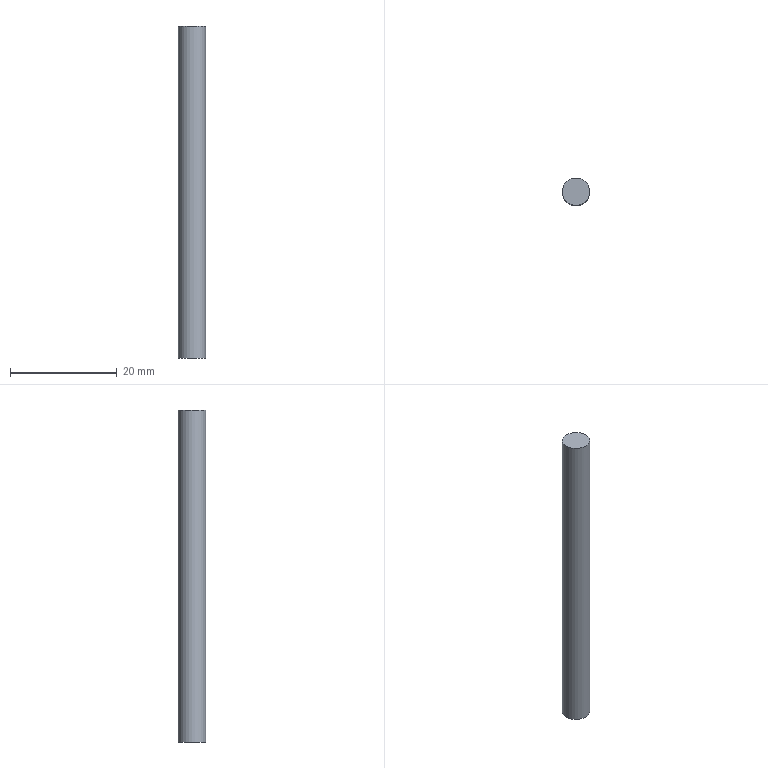Part | STEP file | basic_gh_motor_gh1_03 | 1 solid | 3 faces | box 5.16 x 5.16 x 62.27 mm | volume 1302 mm3 | plane 2 | cylinder 1 | commonest cylinder face diameters 5.16 x1
STEP:
#1=CARTESIAN_POINT('',(-195.92,94.43,107.42));
#2=VERTEX_POINT('',#1);
#3=CARTESIAN_POINT('',(-193.34,94.43,107.42));
#4=DIRECTION('',(0.,0.,1.));
#5=DIRECTION('',(1.,0.,0.));
#6=AXIS2_PLACEMENT_3D('',#3,#4,#5);
#7=CIRCLE('',#6,2.58);
#8=EDGE_CURVE('',#2,#2,#7,.T.);
#9=ORIENTED_EDGE('',*,*,#8,.F.);
#10=CARTESIAN_POINT('',(-195.92,94.43,45.15));
#11=VERTEX_POINT('',#10);
#12=CARTESIAN_POINT('',(-195.92,94.43,76.285));
#13=DIRECTION('',(0.,0.,-1.));
#14=VECTOR('',#13,2.58);
#15=LINE('',#12,#14);
#16=EDGE_CURVE('',#2,#11,#15,.T.);
#17=ORIENTED_EDGE('',*,*,#16,.T.);
#18=CARTESIAN_POINT('',(-193.34,94.43,45.15));
#19=DIRECTION('',(0.,0.,-1.));
#20=DIRECTION('',(1.,0.,0.));
#21=AXIS2_PLACEMENT_3D('',#18,#19,#20);
#22=CIRCLE('',#21,2.58);
#23=EDGE_CURVE('',#11,#11,#22,.T.);
#24=ORIENTED_EDGE('',*,*,#23,.F.);
#25=ORIENTED_EDGE('',*,*,#16,.F.);
#26=EDGE_LOOP('',(#9,#17,#24,#25));
#27=FACE_OUTER_BOUND('',#26,.T.);
#28=CARTESIAN_POINT('',(-193.34,94.43,76.285));
#29=DIRECTION('',(0.,0.,1.));
#30=DIRECTION('',(1.,0.,0.));
#31=AXIS2_PLACEMENT_3D('',#28,#29,#30);
#32=CYLINDRICAL_SURFACE('',#31,2.58);
#33=ADVANCED_FACE('',(#27),#32,.T.);
#34=ORIENTED_EDGE('',*,*,#23,.T.);
#35=EDGE_LOOP('',(#34));
#36=FACE_OUTER_BOUND('',#35,.T.);
#37=CARTESIAN_POINT('',(-193.34,94.43,45.15));
#38=DIRECTION('',(0.,0.,-1.));
#39=DIRECTION('',(-1.,0.,0.));
#40=AXIS2_PLACEMENT_3D('',#37,#38,#39);
#41=PLANE('',#40);
#42=ADVANCED_FACE('',(#36),#41,.T.);
#43=ORIENTED_EDGE('',*,*,#8,.T.);
#44=EDGE_LOOP('',(#43));
#45=FACE_OUTER_BOUND('',#44,.T.);
#46=CARTESIAN_POINT('',(-193.34,94.43,107.42));
#47=DIRECTION('',(0.,0.,1.));
#48=DIRECTION('',(1.,0.,0.));
#49=AXIS2_PLACEMENT_3D('',#46,#47,#48);
#50=PLANE('',#49);
#51=ADVANCED_FACE('',(#45),#50,.T.);
#52=CLOSED_SHELL('',(#33,#42,#51));
#53=MANIFOLD_SOLID_BREP('',#52);
#54=(LENGTH_UNIT()NAMED_UNIT(*)SI_UNIT(.MILLI.,.METRE.));
#55=UNCERTAINTY_MEASURE_WITH_UNIT(LENGTH_MEASURE(0.01),#54,'','');
#56=(NAMED_UNIT(*)PLANE_ANGLE_UNIT()SI_UNIT($,.RADIAN.));
#57=(NAMED_UNIT(*)SI_UNIT($,.STERADIAN.)SOLID_ANGLE_UNIT());
#58=(GEOMETRIC_REPRESENTATION_CONTEXT(3)GLOBAL_UNCERTAINTY_ASSIGNED_CONTEXT((#55))GLOBAL_UNIT_ASSIGNED_CONTEXT((#54,#56,#57))REPRESENTATION_CONTEXT('',''));
#59=ADVANCED_BREP_SHAPE_REPRESENTATION('',(#53),#58);